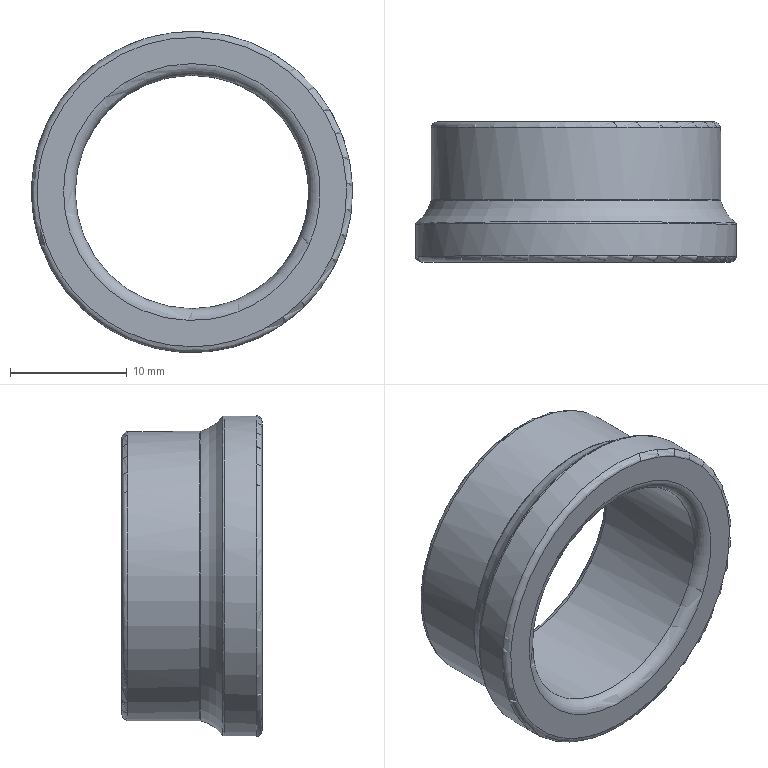Part | STEP file | BK-20_id1250_x_t | 1 solid | 12 faces | box 27.5 x 12 x 27.5 mm | volume 2436 mm3 | torus 7 | cylinder 3 | plane 2 | commonest cylinder face diameters 20 x1 24.8 x1 27.5 x1